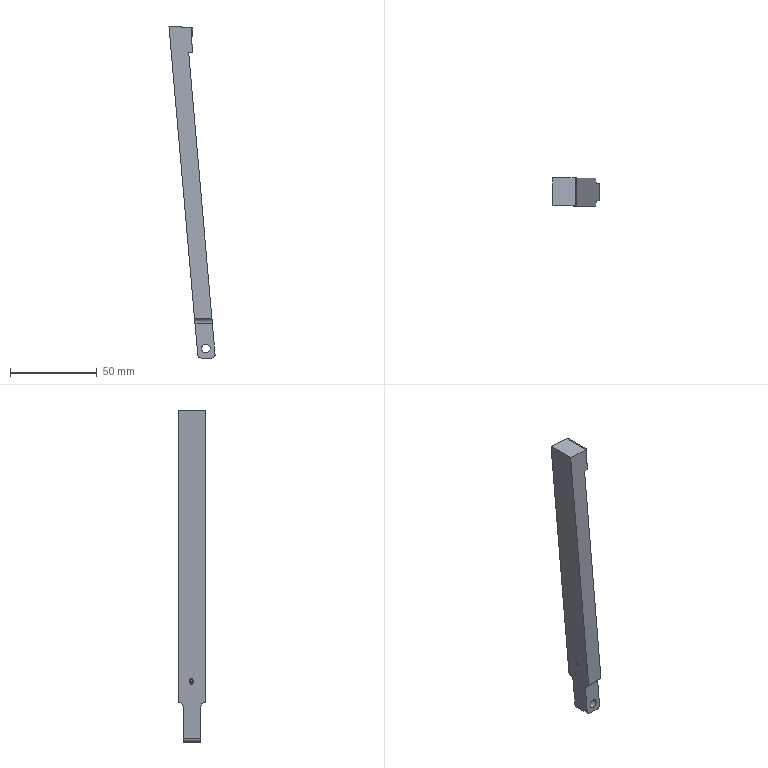Part | STEP file | solid 110 | 1 solid | 29 faces | box 26.632 x 16 x 191.753 mm | volume 29798 mm3 | plane 16 | cylinder 7 | other 4 | spline 2 | commonest cylinder face diameters 4 x2 6 x2 6922 x2 5 x1